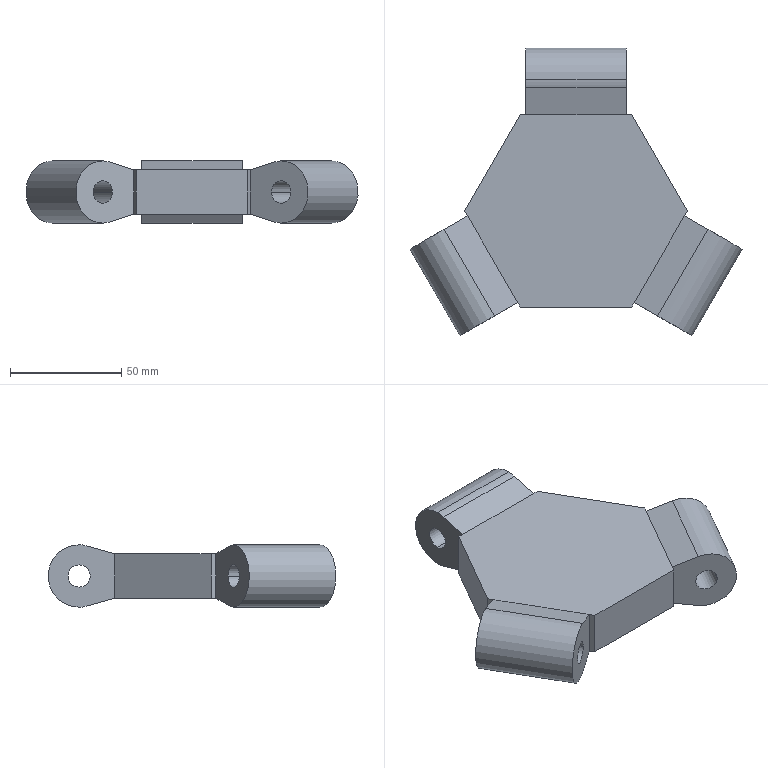Part | SolidWorks | features ICE 2, CirPattern 1, Extrusion 1 | 1 solid | 37 faces | box 149.462 x 129.437 x 28 mm | volume 213673 mm3 | plane 24 | cylinder 13 | commonest cylinder face diameters 10 x8 28 x5
STEP:
#1=CARTESIAN_POINT('',(35.776,-46.636,10.001));
#2=VERTEX_POINT('',#1);
#3=CARTESIAN_POINT('',(44.437,-51.636,10.001));
#4=VERTEX_POINT('',#3);
#5=CARTESIAN_POINT('',(40.106,-49.136,10.001));
#6=DIRECTION('',(-0.5,-0.866,0.));
#7=DIRECTION('',(0.,0.,-1.));
#8=AXIS2_PLACEMENT_3D('',#5,#6,#7);
#9=CIRCLE('',#8,5.);
#10=EDGE_CURVE('',#2,#4,#9,.T.);
#11=ORIENTED_EDGE('',*,*,#10,.T.);
#12=CARTESIAN_POINT('',(66.937,-12.665,10.001));
#13=VERTEX_POINT('',#12);
#14=CARTESIAN_POINT('',(44.437,-51.636,10.001));
#15=DIRECTION('',(0.5,0.866,0.));
#16=VECTOR('',#15,1000.);
#17=LINE('',#14,#16);
#18=EDGE_CURVE('',#4,#13,#17,.T.);
#19=ORIENTED_EDGE('',*,*,#18,.T.);
#20=CARTESIAN_POINT('',(58.276,-7.665,10.001));
#21=VERTEX_POINT('',#20);
#22=CARTESIAN_POINT('',(62.606,-10.165,10.001));
#23=DIRECTION('',(-0.5,-0.866,0.));
#24=DIRECTION('',(0.,0.,-1.));
#25=AXIS2_PLACEMENT_3D('',#22,#23,#24);
#26=CIRCLE('',#25,5.);
#27=EDGE_CURVE('',#21,#13,#26,.T.);
#28=ORIENTED_EDGE('',*,*,#27,.F.);
#29=CARTESIAN_POINT('',(35.776,-46.636,10.001));
#30=DIRECTION('',(0.5,0.866,0.));
#31=VECTOR('',#30,1000.);
#32=LINE('',#29,#31);
#33=EDGE_CURVE('',#2,#21,#32,.T.);
#34=ORIENTED_EDGE('',*,*,#33,.F.);
#35=EDGE_LOOP('',(#11,#19,#28,#34));
#36=FACE_OUTER_BOUND('',#35,.T.);
#37=CARTESIAN_POINT('',(40.106,-49.136,10.001));
#38=DIRECTION('',(0.5,0.866,0.));
#39=DIRECTION('',(-0.866,0.5,0.));
#40=AXIS2_PLACEMENT_3D('',#37,#38,#39);
#41=CYLINDRICAL_SURFACE('',#40,5.);
#42=ADVANCED_FACE('',(#36),#41,.F.);
#43=CARTESIAN_POINT('',(-58.276,-7.665,10.001));
#44=VERTEX_POINT('',#43);
#45=CARTESIAN_POINT('',(-66.937,-12.665,10.001));
#46=VERTEX_POINT('',#45);
#47=CARTESIAN_POINT('',(-62.606,-10.165,10.001));
#48=DIRECTION('',(-0.5,0.866,0.));
#49=DIRECTION('',(0.,0.,-1.));
#50=AXIS2_PLACEMENT_3D('',#47,#48,#49);
#51=CIRCLE('',#50,5.);
#52=EDGE_CURVE('',#44,#46,#51,.T.);
#53=ORIENTED_EDGE('',*,*,#52,.T.);
#54=CARTESIAN_POINT('',(-44.437,-51.636,10.001));
#55=VERTEX_POINT('',#54);
#56=CARTESIAN_POINT('',(-66.937,-12.665,10.001));
#57=DIRECTION('',(0.5,-0.866,0.));
#58=VECTOR('',#57,1000.);
#59=LINE('',#56,#58);
#60=EDGE_CURVE('',#46,#55,#59,.T.);
#61=ORIENTED_EDGE('',*,*,#60,.T.);
#62=CARTESIAN_POINT('',(-35.776,-46.636,10.001));
#63=VERTEX_POINT('',#62);
#64=CARTESIAN_POINT('',(-40.106,-49.136,10.001));
#65=DIRECTION('',(-0.5,0.866,0.));
#66=DIRECTION('',(0.,0.,-1.));
#67=AXIS2_PLACEMENT_3D('',#64,#65,#66);
#68=CIRCLE('',#67,5.);
#69=EDGE_CURVE('',#63,#55,#68,.T.);
#70=ORIENTED_EDGE('',*,*,#69,.F.);
#71=CARTESIAN_POINT('',(-58.276,-7.665,10.001));
#72=DIRECTION('',(0.5,-0.866,0.));
#73=VECTOR('',#72,1000.);
#74=LINE('',#71,#73);
#75=EDGE_CURVE('',#44,#63,#74,.T.);
#76=ORIENTED_EDGE('',*,*,#75,.F.);
#77=EDGE_LOOP('',(#53,#61,#70,#76));
#78=FACE_OUTER_BOUND('',#77,.T.);
#79=CARTESIAN_POINT('',(-62.606,-10.165,10.001));
#80=DIRECTION('',(0.5,-0.866,0.));
#81=DIRECTION('',(0.866,0.5,0.));
#82=AXIS2_PLACEMENT_3D('',#79,#80,#81);
#83=CYLINDRICAL_SURFACE('',#82,5.);
#84=ADVANCED_FACE('',(#78),#83,.F.);
#85=CARTESIAN_POINT('',(5.,0.,0.5));
#86=VERTEX_POINT('',#85);
#87=CARTESIAN_POINT('',(-5.,0.,0.5));
#88=VERTEX_POINT('',#87);
#89=CARTESIAN_POINT('',(0.,0.,0.5));
#90=DIRECTION('',(0.,0.,-1.));
#91=DIRECTION('',(-1.,0.,0.));
#92=AXIS2_PLACEMENT_3D('',#89,#90,#91);
#93=CIRCLE('',#92,5.);
#94=EDGE_CURVE('',#86,#88,#93,.T.);
#95=ORIENTED_EDGE('',*,*,#94,.F.);
#96=CARTESIAN_POINT('',(5.,0.,0.));
#97=VERTEX_POINT('',#96);
#98=CARTESIAN_POINT('',(5.,0.,0.5));
#99=DIRECTION('',(0.,0.,-1.));
#100=VECTOR('',#99,1000.);
#101=LINE('',#98,#100);
#102=EDGE_CURVE('',#86,#97,#101,.T.);
#103=ORIENTED_EDGE('',*,*,#102,.T.);
#104=CARTESIAN_POINT('',(-5.,0.,0.));
#105=VERTEX_POINT('',#104);
#106=CARTESIAN_POINT('',(0.,0.,0.));
#107=DIRECTION('',(0.,0.,-1.));
#108=DIRECTION('',(-1.,0.,0.));
#109=AXIS2_PLACEMENT_3D('',#106,#107,#108);
#110=CIRCLE('',#109,5.);
#111=EDGE_CURVE('',#97,#105,#110,.T.);
#112=ORIENTED_EDGE('',*,*,#111,.T.);
#113=CARTESIAN_POINT('',(-5.,0.,0.5));
#114=DIRECTION('',(0.,0.,-1.));
#115=VECTOR('',#114,1000.);
#116=LINE('',#113,#115);
#117=EDGE_CURVE('',#88,#105,#116,.T.);
#118=ORIENTED_EDGE('',*,*,#117,.F.);
#119=EDGE_LOOP('',(#95,#103,#112,#118));
#120=FACE_OUTER_BOUND('',#119,.T.);
#121=CARTESIAN_POINT('',(0.,0.,0.5));
#122=DIRECTION('',(0.,0.,-1.));
#123=DIRECTION('',(-1.,0.,0.));
#124=AXIS2_PLACEMENT_3D('',#121,#122,#123);
#125=CYLINDRICAL_SURFACE('',#124,5.);
#126=ADVANCED_FACE('',(#120),#125,.F.);
#127=CARTESIAN_POINT('',(22.5,59.301,15.001));
#128=VERTEX_POINT('',#127);
#129=CARTESIAN_POINT('',(22.5,59.301,5.001));
#130=VERTEX_POINT('',#129);
#131=CARTESIAN_POINT('',(22.5,59.301,10.001));
#132=DIRECTION('',(1.,0.,0.));
#133=DIRECTION('',(0.,0.,-1.));
#134=AXIS2_PLACEMENT_3D('',#131,#132,#133);
#135=CIRCLE('',#134,5.);
#136=EDGE_CURVE('',#128,#130,#135,.T.);
#137=ORIENTED_EDGE('',*,*,#136,.T.);
#138=CARTESIAN_POINT('',(-22.5,59.301,5.001));
#139=VERTEX_POINT('',#138);
#140=CARTESIAN_POINT('',(22.5,59.301,5.001));
#141=DIRECTION('',(-1.,0.,0.));
#142=VECTOR('',#141,1000.);
#143=LINE('',#140,#142);
#144=EDGE_CURVE('',#130,#139,#143,.T.);
#145=ORIENTED_EDGE('',*,*,#144,.T.);
#146=CARTESIAN_POINT('',(-22.5,59.301,15.001));
#147=VERTEX_POINT('',#146);
#148=CARTESIAN_POINT('',(-22.5,59.301,10.001));
#149=DIRECTION('',(1.,0.,0.));
#150=DIRECTION('',(0.,0.,-1.));
#151=AXIS2_PLACEMENT_3D('',#148,#149,#150);
#152=CIRCLE('',#151,5.);
#153=EDGE_CURVE('',#147,#139,#152,.T.);
#154=ORIENTED_EDGE('',*,*,#153,.F.);
#155=CARTESIAN_POINT('',(22.5,59.301,15.001));
#156=DIRECTION('',(-1.,0.,0.));
#157=VECTOR('',#156,1000.);
#158=LINE('',#155,#157);
#159=EDGE_CURVE('',#128,#147,#158,.T.);
#160=ORIENTED_EDGE('',*,*,#159,.F.);
#161=EDGE_LOOP('',(#137,#145,#154,#160));
#162=FACE_OUTER_BOUND('',#161,.T.);
#163=CARTESIAN_POINT('',(22.5,59.301,10.001));
#164=DIRECTION('',(-1.,0.,0.));
#165=DIRECTION('',(0.,0.,1.));
#166=AXIS2_PLACEMENT_3D('',#163,#164,#165);
#167=CYLINDRICAL_SURFACE('',#166,5.);
#168=ADVANCED_FACE('',(#162),#167,.F.);
#169=CARTESIAN_POINT('',(22.5,59.301,-3.999));
#170=VERTEX_POINT('',#169);
#171=CARTESIAN_POINT('',(22.5,59.301,24.001));
#172=VERTEX_POINT('',#171);
#173=CARTESIAN_POINT('',(22.5,59.301,10.001));
#174=DIRECTION('',(1.,0.,0.));
#175=DIRECTION('',(0.,0.,-1.));
#176=AXIS2_PLACEMENT_3D('',#173,#174,#175);
#177=CIRCLE('',#176,14.);
#178=EDGE_CURVE('',#170,#172,#177,.T.);
#179=ORIENTED_EDGE('',*,*,#178,.F.);
#180=CARTESIAN_POINT('',(-22.5,59.301,-3.999));
#181=VERTEX_POINT('',#180);
#182=CARTESIAN_POINT('',(22.5,59.301,-3.999));
#183=DIRECTION('',(-1.,0.,0.));
#184=VECTOR('',#183,1000.);
#185=LINE('',#182,#184);
#186=EDGE_CURVE('',#170,#181,#185,.T.);
#187=ORIENTED_EDGE('',*,*,#186,.T.);
#188=CARTESIAN_POINT('',(-22.5,59.301,24.001));
#189=VERTEX_POINT('',#188);
#190=CARTESIAN_POINT('',(-22.5,59.301,10.001));
#191=DIRECTION('',(1.,0.,0.));
#192=DIRECTION('',(0.,0.,-1.));
#193=AXIS2_PLACEMENT_3D('',#190,#191,#192);
#194=CIRCLE('',#193,14.);
#195=EDGE_CURVE('',#181,#189,#194,.T.);
#196=ORIENTED_EDGE('',*,*,#195,.T.);
#197=CARTESIAN_POINT('',(22.5,59.301,24.001));
#198=DIRECTION('',(-1.,0.,0.));
#199=VECTOR('',#198,1000.);
#200=LINE('',#197,#199);
#201=EDGE_CURVE('',#172,#189,#200,.T.);
#202=ORIENTED_EDGE('',*,*,#201,.F.);
#203=EDGE_LOOP('',(#179,#187,#196,#202));
#204=FACE_OUTER_BOUND('',#203,.T.);
#205=CARTESIAN_POINT('',(22.5,59.301,10.001));
#206=DIRECTION('',(-1.,0.,0.));
#207=DIRECTION('',(0.,0.,1.));
#208=AXIS2_PLACEMENT_3D('',#205,#206,#207);
#209=CYLINDRICAL_SURFACE('',#208,14.);
#210=ADVANCED_FACE('',(#204),#209,.T.);
#211=CARTESIAN_POINT('',(22.5,55.466,23.465));
#212=VERTEX_POINT('',#211);
#213=CARTESIAN_POINT('',(22.5,59.301,10.001));
#214=DIRECTION('',(1.,0.,0.));
#215=DIRECTION('',(0.,0.,-1.));
#216=AXIS2_PLACEMENT_3D('',#213,#214,#215);
#217=CIRCLE('',#216,14.);
#218=EDGE_CURVE('',#172,#212,#217,.T.);
#219=ORIENTED_EDGE('',*,*,#218,.F.);
#220=ORIENTED_EDGE('',*,*,#201,.T.);
#221=CARTESIAN_POINT('',(-22.5,55.466,23.465));
#222=VERTEX_POINT('',#221);
#223=CARTESIAN_POINT('',(-22.5,59.301,10.001));
#224=DIRECTION('',(1.,0.,0.));
#225=DIRECTION('',(0.,0.,-1.));
#226=AXIS2_PLACEMENT_3D('',#223,#224,#225);
#227=CIRCLE('',#226,14.);
#228=EDGE_CURVE('',#189,#222,#227,.T.);
#229=ORIENTED_EDGE('',*,*,#228,.T.);
#230=CARTESIAN_POINT('',(22.5,55.466,23.465));
#231=DIRECTION('',(-1.,0.,0.));
#232=VECTOR('',#231,1000.);
#233=LINE('',#230,#232);
#234=EDGE_CURVE('',#212,#222,#233,.T.);
#235=ORIENTED_EDGE('',*,*,#234,.F.);
#236=EDGE_LOOP('',(#219,#220,#229,#235));
#237=FACE_OUTER_BOUND('',#236,.T.);
#238=CARTESIAN_POINT('',(22.5,59.301,10.001));
#239=DIRECTION('',(-1.,0.,0.));
#240=DIRECTION('',(0.,0.,1.));
#241=AXIS2_PLACEMENT_3D('',#238,#239,#240);
#242=CYLINDRICAL_SURFACE('',#241,14.);
#243=ADVANCED_FACE('',(#237),#242,.T.);
#244=CARTESIAN_POINT('',(48.75,-2.165,20.));
#245=VERTEX_POINT('',#244);
#246=CARTESIAN_POINT('',(48.75,-2.165,0.));
#247=VERTEX_POINT('',#246);
#248=CARTESIAN_POINT('',(48.75,-2.165,20.));
#249=DIRECTION('',(0.,0.,-1.));
#250=VECTOR('',#249,1000.);
#251=LINE('',#248,#250);
#252=EDGE_CURVE('',#245,#247,#251,.T.);
#253=ORIENTED_EDGE('',*,*,#252,.T.);
#254=CARTESIAN_POINT('',(50.,0.,0.));
#255=VERTEX_POINT('',#254);
#256=CARTESIAN_POINT('',(25.,-43.301,0.));
#257=DIRECTION('',(0.5,0.866,0.));
#258=VECTOR('',#257,1000.);
#259=LINE('',#256,#258);
#260=EDGE_CURVE('',#247,#255,#259,.T.);
#261=ORIENTED_EDGE('',*,*,#260,.T.);
#262=CARTESIAN_POINT('',(50.,0.,20.));
#263=VERTEX_POINT('',#262);
#264=CARTESIAN_POINT('',(50.,0.,20.));
#265=DIRECTION('',(0.,0.,-1.));
#266=VECTOR('',#265,1000.);
#267=LINE('',#264,#266);
#268=EDGE_CURVE('',#263,#255,#267,.T.);
#269=ORIENTED_EDGE('',*,*,#268,.F.);
#270=CARTESIAN_POINT('',(25.,-43.301,20.));
#271=DIRECTION('',(0.5,0.866,0.));
#272=VECTOR('',#271,1000.);
#273=LINE('',#270,#272);
#274=EDGE_CURVE('',#245,#263,#273,.T.);
#275=ORIENTED_EDGE('',*,*,#274,.F.);
#276=EDGE_LOOP('',(#253,#261,#269,#275));
#277=FACE_OUTER_BOUND('',#276,.T.);
#278=CARTESIAN_POINT('',(25.,-43.301,20.));
#279=DIRECTION('',(-0.866,0.5,0.));
#280=DIRECTION('',(-0.5,-0.866,0.));
#281=AXIS2_PLACEMENT_3D('',#278,#279,#280);
#282=PLANE('',#281);
#283=ADVANCED_FACE('',(#277),#282,.F.);
#284=CARTESIAN_POINT('',(-26.25,-41.136,20.));
#285=VERTEX_POINT('',#284);
#286=CARTESIAN_POINT('',(-26.25,-41.136,0.));
#287=VERTEX_POINT('',#286);
#288=CARTESIAN_POINT('',(-26.25,-41.136,20.));
#289=DIRECTION('',(0.,0.,-1.));
#290=VECTOR('',#289,1000.);
#291=LINE('',#288,#290);
#292=EDGE_CURVE('',#285,#287,#291,.T.);
#293=ORIENTED_EDGE('',*,*,#292,.T.);
#294=CARTESIAN_POINT('',(-25.,-43.301,0.));
#295=VERTEX_POINT('',#294);
#296=CARTESIAN_POINT('',(-50.,0.,0.));
#297=DIRECTION('',(0.5,-0.866,0.));
#298=VECTOR('',#297,1000.);
#299=LINE('',#296,#298);
#300=EDGE_CURVE('',#287,#295,#299,.T.);
#301=ORIENTED_EDGE('',*,*,#300,.T.);
#302=CARTESIAN_POINT('',(-25.,-43.301,20.));
#303=VERTEX_POINT('',#302);
#304=CARTESIAN_POINT('',(-25.,-43.301,20.));
#305=DIRECTION('',(0.,0.,-1.));
#306=VECTOR('',#305,1000.);
#307=LINE('',#304,#306);
#308=EDGE_CURVE('',#303,#295,#307,.T.);
#309=ORIENTED_EDGE('',*,*,#308,.F.);
#310=CARTESIAN_POINT('',(-50.,0.,20.));
#311=DIRECTION('',(0.5,-0.866,0.));
#312=VECTOR('',#311,1000.);
#313=LINE('',#310,#312);
#314=EDGE_CURVE('',#285,#303,#313,.T.);
#315=ORIENTED_EDGE('',*,*,#314,.F.);
#316=EDGE_LOOP('',(#293,#301,#309,#315));
#317=FACE_OUTER_BOUND('',#316,.T.);
#318=CARTESIAN_POINT('',(-50.,0.,20.));
#319=DIRECTION('',(0.866,0.5,0.));
#320=DIRECTION('',(-0.5,0.866,0.));
#321=AXIS2_PLACEMENT_3D('',#318,#319,#320);
#322=PLANE('',#321);
#323=ADVANCED_FACE('',(#317),#322,.F.);
#324=CARTESIAN_POINT('',(22.5,43.301,20.));
#325=VERTEX_POINT('',#324);
#326=CARTESIAN_POINT('',(22.5,43.301,0.));
#327=VERTEX_POINT('',#326);
#328=CARTESIAN_POINT('',(22.5,43.301,20.));
#329=DIRECTION('',(0.,0.,-1.));
#330=VECTOR('',#329,1000.);
#331=LINE('',#328,#330);
#332=EDGE_CURVE('',#325,#327,#331,.T.);
#333=ORIENTED_EDGE('',*,*,#332,.F.);
#334=CARTESIAN_POINT('',(25.,43.301,20.));
#335=VERTEX_POINT('',#334);
#336=CARTESIAN_POINT('',(25.,43.301,20.));
#337=DIRECTION('',(-1.,0.,0.));
#338=VECTOR('',#337,1000.);
#339=LINE('',#336,#338);
#340=EDGE_CURVE('',#335,#325,#339,.T.);
#341=ORIENTED_EDGE('',*,*,#340,.F.);
#342=CARTESIAN_POINT('',(25.,43.301,0.));
#343=VERTEX_POINT('',#342);
#344=CARTESIAN_POINT('',(25.,43.301,20.));
#345=DIRECTION('',(0.,0.,-1.));
#346=VECTOR('',#345,1000.);
#347=LINE('',#344,#346);
#348=EDGE_CURVE('',#335,#343,#347,.T.);
#349=ORIENTED_EDGE('',*,*,#348,.T.);
#350=CARTESIAN_POINT('',(25.,43.301,0.));
#351=DIRECTION('',(-1.,0.,0.));
#352=VECTOR('',#351,1000.);
#353=LINE('',#350,#352);
#354=EDGE_CURVE('',#343,#327,#353,.T.);
#355=ORIENTED_EDGE('',*,*,#354,.T.);
#356=EDGE_LOOP('',(#333,#341,#349,#355));
#357=FACE_OUTER_BOUND('',#356,.T.);
#358=CARTESIAN_POINT('',(25.,43.301,20.));
#359=DIRECTION('',(0.,-1.,0.));
#360=DIRECTION('',(1.,0.,0.));
#361=AXIS2_PLACEMENT_3D('',#358,#359,#360);
#362=PLANE('',#361);
#363=ADVANCED_FACE('',(#357),#362,.F.);
#364=CARTESIAN_POINT('',(25.,-43.301,0.));
#365=VERTEX_POINT('',#364);
#366=CARTESIAN_POINT('',(26.25,-41.136,0.));
#367=VERTEX_POINT('',#366);
#368=CARTESIAN_POINT('',(25.,-43.301,0.));
#369=DIRECTION('',(0.5,0.866,0.));
#370=VECTOR('',#369,1000.);
#371=LINE('',#368,#370);
#372=EDGE_CURVE('',#365,#367,#371,.T.);
#373=ORIENTED_EDGE('',*,*,#372,.T.);
#374=CARTESIAN_POINT('',(26.25,-41.136,20.));
#375=VERTEX_POINT('',#374);
#376=CARTESIAN_POINT('',(26.25,-41.136,20.));
#377=DIRECTION('',(0.,0.,-1.));
#378=VECTOR('',#377,1000.);
#379=LINE('',#376,#378);
#380=EDGE_CURVE('',#375,#367,#379,.T.);
#381=ORIENTED_EDGE('',*,*,#380,.F.);
#382=CARTESIAN_POINT('',(25.,-43.301,20.));
#383=VERTEX_POINT('',#382);
#384=CARTESIAN_POINT('',(25.,-43.301,20.));
#385=DIRECTION('',(0.5,0.866,0.));
#386=VECTOR('',#385,1000.);
#387=LINE('',#384,#386);
#388=EDGE_CURVE('',#383,#375,#387,.T.);
#389=ORIENTED_EDGE('',*,*,#388,.F.);
#390=CARTESIAN_POINT('',(25.,-43.301,20.));
#391=DIRECTION('',(0.,0.,-1.));
#392=VECTOR('',#391,1000.);
#393=LINE('',#390,#392);
#394=EDGE_CURVE('',#383,#365,#393,.T.);
#395=ORIENTED_EDGE('',*,*,#394,.T.);
#396=EDGE_LOOP('',(#373,#381,#389,#395));
#397=FACE_OUTER_BOUND('',#396,.T.);
#398=CARTESIAN_POINT('',(25.,-43.301,20.));
#399=DIRECTION('',(-0.866,0.5,0.));
#400=DIRECTION('',(-0.5,-0.866,0.));
#401=AXIS2_PLACEMENT_3D('',#398,#399,#400);
#402=PLANE('',#401);
#403=ADVANCED_FACE('',(#397),#402,.F.);
#404=CARTESIAN_POINT('',(50.,0.,0.));
#405=DIRECTION('',(-0.5,0.866,0.));
#406=VECTOR('',#405,1000.);
#407=LINE('',#404,#406);
#408=EDGE_CURVE('',#255,#343,#407,.T.);
#409=ORIENTED_EDGE('',*,*,#408,.T.);
#410=ORIENTED_EDGE('',*,*,#348,.F.);
#411=CARTESIAN_POINT('',(50.,0.,20.));
#412=DIRECTION('',(-0.5,0.866,0.));
#413=VECTOR('',#412,1000.);
#414=LINE('',#411,#413);
#415=EDGE_CURVE('',#263,#335,#414,.T.);
#416=ORIENTED_EDGE('',*,*,#415,.F.);
#417=ORIENTED_EDGE('',*,*,#268,.T.);
#418=EDGE_LOOP('',(#409,#410,#416,#417));
#419=FACE_OUTER_BOUND('',#418,.T.);
#420=CARTESIAN_POINT('',(50.,0.,20.));
#421=DIRECTION('',(-0.866,-0.5,0.));
#422=DIRECTION('',(0.5,-0.866,0.));
#423=AXIS2_PLACEMENT_3D('',#420,#421,#422);
#424=PLANE('',#423);
#425=ADVANCED_FACE('',(#419),#424,.F.);
#426=CARTESIAN_POINT('',(-22.5,43.301,20.));
#427=VERTEX_POINT('',#426);
#428=CARTESIAN_POINT('',(-25.,43.301,20.));
#429=VERTEX_POINT('',#428);
#430=CARTESIAN_POINT('',(25.,43.301,20.));
#431=DIRECTION('',(-1.,0.,0.));
#432=VECTOR('',#431,1000.);
#433=LINE('',#430,#432);
#434=EDGE_CURVE('',#427,#429,#433,.T.);
#435=ORIENTED_EDGE('',*,*,#434,.F.);
#436=CARTESIAN_POINT('',(-22.5,43.301,0.));
#437=VERTEX_POINT('',#436);
#438=CARTESIAN_POINT('',(-22.5,43.301,20.));
#439=DIRECTION('',(0.,0.,-1.));
#440=VECTOR('',#439,1000.);
#441=LINE('',#438,#440);
#442=EDGE_CURVE('',#427,#437,#441,.T.);
#443=ORIENTED_EDGE('',*,*,#442,.T.);
#444=CARTESIAN_POINT('',(-25.,43.301,0.));
#445=VERTEX_POINT('',#444);
#446=CARTESIAN_POINT('',(25.,43.301,0.));
#447=DIRECTION('',(-1.,0.,0.));
#448=VECTOR('',#447,1000.);
#449=LINE('',#446,#448);
#450=EDGE_CURVE('',#437,#445,#449,.T.);
#451=ORIENTED_EDGE('',*,*,#450,.T.);
#452=CARTESIAN_POINT('',(-25.,43.301,20.));
#453=DIRECTION('',(0.,0.,-1.));
#454=VECTOR('',#453,1000.);
#455=LINE('',#452,#454);
#456=EDGE_CURVE('',#429,#445,#455,.T.);
#457=ORIENTED_EDGE('',*,*,#456,.F.);
#458=EDGE_LOOP('',(#435,#443,#451,#457));
#459=FACE_OUTER_BOUND('',#458,.T.);
#460=CARTESIAN_POINT('',(25.,43.301,20.));
#461=DIRECTION('',(0.,-1.,0.));
#462=DIRECTION('',(1.,0.,0.));
#463=AXIS2_PLACEMENT_3D('',#460,#461,#462);
#464=PLANE('',#463);
#465=ADVANCED_FACE('',(#459),#464,.F.);
#466=CARTESIAN_POINT('',(-50.,0.,0.));
#467=VERTEX_POINT('',#466);
#468=CARTESIAN_POINT('',(-25.,43.301,0.));
#469=DIRECTION('',(-0.5,-0.866,0.));
#470=VECTOR('',#469,1000.);
#471=LINE('',#468,#470);
#472=EDGE_CURVE('',#445,#467,#471,.T.);
#473=ORIENTED_EDGE('',*,*,#472,.T.);
#474=CARTESIAN_POINT('',(-50.,0.,20.));
#475=VERTEX_POINT('',#474);
#476=CARTESIAN_POINT('',(-50.,0.,20.));
#477=DIRECTION('',(0.,0.,-1.));
#478=VECTOR('',#477,1000.);
#479=LINE('',#476,#478);
#480=EDGE_CURVE('',#475,#467,#479,.T.);
#481=ORIENTED_EDGE('',*,*,#480,.F.);
#482=CARTESIAN_POINT('',(-25.,43.301,20.));
#483=DIRECTION('',(-0.5,-0.866,0.));
#484=VECTOR('',#483,1000.);
#485=LINE('',#482,#484);
#486=EDGE_CURVE('',#429,#475,#485,.T.);
#487=ORIENTED_EDGE('',*,*,#486,.F.);
#488=ORIENTED_EDGE('',*,*,#456,.T.);
#489=EDGE_LOOP('',(#473,#481,#487,#488));
#490=FACE_OUTER_BOUND('',#489,.T.);
#491=CARTESIAN_POINT('',(-25.,43.301,20.));
#492=DIRECTION('',(0.866,-0.5,0.));
#493=DIRECTION('',(0.5,0.866,0.));
#494=AXIS2_PLACEMENT_3D('',#491,#492,#493);
#495=PLANE('',#494);
#496=ADVANCED_FACE('',(#490),#495,.F.);
#497=CARTESIAN_POINT('',(-48.75,-2.165,0.));
#498=VERTEX_POINT('',#497);
#499=CARTESIAN_POINT('',(-50.,0.,0.));
#500=DIRECTION('',(0.5,-0.866,0.));
#501=VECTOR('',#500,1000.);
#502=LINE('',#499,#501);
#503=EDGE_CURVE('',#467,#498,#502,.T.);
#504=ORIENTED_EDGE('',*,*,#503,.T.);
#505=CARTESIAN_POINT('',(-48.75,-2.165,20.));
#506=VERTEX_POINT('',#505);
#507=CARTESIAN_POINT('',(-48.75,-2.165,20.));
#508=DIRECTION('',(0.,0.,-1.));
#509=VECTOR('',#508,1000.);
#510=LINE('',#507,#509);
#511=EDGE_CURVE('',#506,#498,#510,.T.);
#512=ORIENTED_EDGE('',*,*,#511,.F.);
#513=CARTESIAN_POINT('',(-50.,0.,20.));
#514=DIRECTION('',(0.5,-0.866,0.));
#515=VECTOR('',#514,1000.);
#516=LINE('',#513,#515);
#517=EDGE_CURVE('',#475,#506,#516,.T.);
#518=ORIENTED_EDGE('',*,*,#517,.F.);
#519=ORIENTED_EDGE('',*,*,#480,.T.);
#520=EDGE_LOOP('',(#504,#512,#518,#519));
#521=FACE_OUTER_BOUND('',#520,.T.);
#522=CARTESIAN_POINT('',(-50.,0.,20.));
#523=DIRECTION('',(0.866,0.5,0.));
#524=DIRECTION('',(-0.5,0.866,0.));
#525=AXIS2_PLACEMENT_3D('',#522,#523,#524);
#526=PLANE('',#525);
#527=ADVANCED_FACE('',(#521),#526,.F.);
#528=CARTESIAN_POINT('',(-25.,-43.301,0.));
#529=DIRECTION('',(1.,0.,0.));
#530=VECTOR('',#529,1000.);
#531=LINE('',#528,#530);
#532=EDGE_CURVE('',#295,#365,#531,.T.);
#533=ORIENTED_EDGE('',*,*,#532,.T.);
#534=ORIENTED_EDGE('',*,*,#394,.F.);
#535=CARTESIAN_POINT('',(-25.,-43.301,20.));
#536=DIRECTION('',(1.,0.,0.));
#537=VECTOR('',#536,1000.);
#538=LINE('',#535,#537);
#539=EDGE_CURVE('',#303,#383,#538,.T.);
#540=ORIENTED_EDGE('',*,*,#539,.F.);
#541=ORIENTED_EDGE('',*,*,#308,.T.);
#542=EDGE_LOOP('',(#533,#534,#540,#541));
#543=FACE_OUTER_BOUND('',#542,.T.);
#544=CARTESIAN_POINT('',(-25.,-43.301,20.));
#545=DIRECTION('',(0.,1.,0.));
#546=DIRECTION('',(-1.,0.,0.));
#547=AXIS2_PLACEMENT_3D('',#544,#545,#546);
#548=PLANE('',#547);
#549=ADVANCED_FACE('',(#543),#548,.F.);
#550=ORIENTED_EDGE('',*,*,#388,.T.);
#551=CARTESIAN_POINT('',(26.25,-41.136,20.));
#552=DIRECTION('',(0.5,0.866,0.));
#553=VECTOR('',#552,1000.);
#554=LINE('',#551,#553);
#555=EDGE_CURVE('',#375,#245,#554,.T.);
#556=ORIENTED_EDGE('',*,*,#555,.T.);
#557=ORIENTED_EDGE('',*,*,#274,.T.);
#558=ORIENTED_EDGE('',*,*,#415,.T.);
#559=ORIENTED_EDGE('',*,*,#340,.T.);
#560=CARTESIAN_POINT('',(22.5,43.301,20.));
#561=DIRECTION('',(-1.,0.,0.));
#562=VECTOR('',#561,1000.);
#563=LINE('',#560,#562);
#564=EDGE_CURVE('',#325,#427,#563,.T.);
#565=ORIENTED_EDGE('',*,*,#564,.T.);
#566=ORIENTED_EDGE('',*,*,#434,.T.);
#567=ORIENTED_EDGE('',*,*,#486,.T.);
#568=ORIENTED_EDGE('',*,*,#517,.T.);
#569=CARTESIAN_POINT('',(-48.75,-2.165,20.));
#570=DIRECTION('',(0.5,-0.866,0.));
#571=VECTOR('',#570,1000.);
#572=LINE('',#569,#571);
#573=EDGE_CURVE('',#506,#285,#572,.T.);
#574=ORIENTED_EDGE('',*,*,#573,.T.);
#575=ORIENTED_EDGE('',*,*,#314,.T.);
#576=ORIENTED_EDGE('',*,*,#539,.T.);
#577=EDGE_LOOP('',(#550,#556,#557,#558,#559,#565,#566,#567,#568,#574,#575,#576));
#578=FACE_OUTER_BOUND('',#577,.T.);
#579=CARTESIAN_POINT('',(0.,0.,20.));
#580=DIRECTION('',(0.,0.,1.));
#581=DIRECTION('',(1.,0.,0.));
#582=AXIS2_PLACEMENT_3D('',#579,#580,#581);
#583=PLANE('',#582);
#584=ADVANCED_FACE('',(#578),#583,.T.);
#585=CARTESIAN_POINT('',(0.,0.,0.));
#586=DIRECTION('',(0.,0.,-1.));
#587=DIRECTION('',(-1.,0.,0.));
#588=AXIS2_PLACEMENT_3D('',#585,#586,#587);
#589=CIRCLE('',#588,5.);
#590=EDGE_CURVE('',#105,#97,#589,.T.);
#591=ORIENTED_EDGE('',*,*,#590,.F.);
#592=ORIENTED_EDGE('',*,*,#111,.F.);
#593=EDGE_LOOP('',(#591,#592));
#594=FACE_BOUND('',#593,.T.);
#595=ORIENTED_EDGE('',*,*,#372,.F.);
#596=ORIENTED_EDGE('',*,*,#532,.F.);
#597=ORIENTED_EDGE('',*,*,#300,.F.);
#598=CARTESIAN_POINT('',(-48.75,-2.165,0.));
#599=DIRECTION('',(0.5,-0.866,0.));
#600=VECTOR('',#599,1000.);
#601=LINE('',#598,#600);
#602=EDGE_CURVE('',#498,#287,#601,.T.);
#603=ORIENTED_EDGE('',*,*,#602,.F.);
#604=ORIENTED_EDGE('',*,*,#503,.F.);
#605=ORIENTED_EDGE('',*,*,#472,.F.);
#606=ORIENTED_EDGE('',*,*,#450,.F.);
#607=CARTESIAN_POINT('',(22.5,43.301,0.));
#608=DIRECTION('',(-1.,0.,0.));
#609=VECTOR('',#608,1000.);
#610=LINE('',#607,#609);
#611=EDGE_CURVE('',#327,#437,#610,.T.);
#612=ORIENTED_EDGE('',*,*,#611,.F.);
#613=ORIENTED_EDGE('',*,*,#354,.F.);
#614=ORIENTED_EDGE('',*,*,#408,.F.);
#615=ORIENTED_EDGE('',*,*,#260,.F.);
#616=CARTESIAN_POINT('',(26.25,-41.136,0.));
#617=DIRECTION('',(0.5,0.866,0.));
#618=VECTOR('',#617,1000.);
#619=LINE('',#616,#618);
#620=EDGE_CURVE('',#367,#247,#619,.T.);
#621=ORIENTED_EDGE('',*,*,#620,.F.);
#622=EDGE_LOOP('',(#595,#596,#597,#603,#604,#605,#606,#612,#613,#614,#615,#621));
#623=FACE_OUTER_BOUND('',#622,.T.);
#624=CARTESIAN_POINT('',(0.,0.,0.));
#625=DIRECTION('',(0.,0.,1.));
#626=DIRECTION('',(1.,0.,0.));
#627=AXIS2_PLACEMENT_3D('',#624,#625,#626);
#628=PLANE('',#627);
#629=ADVANCED_FACE('',(#594,#623),#628,.F.);
#630=ORIENTED_EDGE('',*,*,#332,.T.);
#631=CARTESIAN_POINT('',(22.5,55.467,-3.464));
#632=VERTEX_POINT('',#631);
#633=CARTESIAN_POINT('',(22.5,43.301,0.));
#634=DIRECTION('',(0.,0.9618,-0.2738));
#635=VECTOR('',#634,1000.);
#636=LINE('',#633,#635);
#637=EDGE_CURVE('',#327,#632,#636,.T.);
#638=ORIENTED_EDGE('',*,*,#637,.T.);
#639=CARTESIAN_POINT('',(22.5,59.301,10.001));
#640=DIRECTION('',(1.,0.,0.));
#641=DIRECTION('',(0.,0.,-1.));
#642=AXIS2_PLACEMENT_3D('',#639,#640,#641);
#643=CIRCLE('',#642,14.);
#644=EDGE_CURVE('',#632,#170,#643,.T.);
#645=ORIENTED_EDGE('',*,*,#644,.T.);
#646=ORIENTED_EDGE('',*,*,#178,.T.);
#647=ORIENTED_EDGE('',*,*,#218,.T.);
#648=CARTESIAN_POINT('',(22.5,43.301,20.));
#649=DIRECTION('',(0.,-0.9617,-0.274));
#650=VECTOR('',#649,1000.);
#651=LINE('',#648,#650);
#652=EDGE_CURVE('',#212,#325,#651,.T.);
#653=ORIENTED_EDGE('',*,*,#652,.T.);
#654=EDGE_LOOP('',(#630,#638,#645,#646,#647,#653));
#655=FACE_OUTER_BOUND('',#654,.T.);
#656=ORIENTED_EDGE('',*,*,#136,.F.);
#657=CARTESIAN_POINT('',(22.5,59.301,10.001));
#658=DIRECTION('',(1.,0.,0.));
#659=DIRECTION('',(0.,0.,-1.));
#660=AXIS2_PLACEMENT_3D('',#657,#658,#659);
#661=CIRCLE('',#660,5.);
#662=EDGE_CURVE('',#130,#128,#661,.T.);
#663=ORIENTED_EDGE('',*,*,#662,.F.);
#664=EDGE_LOOP('',(#656,#663));
#665=FACE_BOUND('',#664,.T.);
#666=CARTESIAN_POINT('',(22.5,59.301,10.001));
#667=DIRECTION('',(1.,0.,0.));
#668=DIRECTION('',(0.,0.,-1.));
#669=AXIS2_PLACEMENT_3D('',#666,#667,#668);
#670=PLANE('',#669);
#671=ADVANCED_FACE('',(#655,#665),#670,.T.);
#672=ORIENTED_EDGE('',*,*,#442,.F.);
#673=CARTESIAN_POINT('',(-22.5,43.301,20.));
#674=DIRECTION('',(0.,-0.9617,-0.274));
#675=VECTOR('',#674,1000.);
#676=LINE('',#673,#675);
#677=EDGE_CURVE('',#222,#427,#676,.T.);
#678=ORIENTED_EDGE('',*,*,#677,.F.);
#679=ORIENTED_EDGE('',*,*,#228,.F.);
#680=ORIENTED_EDGE('',*,*,#195,.F.);
#681=CARTESIAN_POINT('',(-22.5,55.467,-3.464));
#682=VERTEX_POINT('',#681);
#683=CARTESIAN_POINT('',(-22.5,59.301,10.001));
#684=DIRECTION('',(1.,0.,0.));
#685=DIRECTION('',(0.,0.,-1.));
#686=AXIS2_PLACEMENT_3D('',#683,#684,#685);
#687=CIRCLE('',#686,14.);
#688=EDGE_CURVE('',#682,#181,#687,.T.);
#689=ORIENTED_EDGE('',*,*,#688,.F.);
#690=CARTESIAN_POINT('',(-22.5,43.301,0.));
#691=DIRECTION('',(0.,0.9618,-0.2738));
#692=VECTOR('',#691,1000.);
#693=LINE('',#690,#692);
#694=EDGE_CURVE('',#437,#682,#693,.T.);
#695=ORIENTED_EDGE('',*,*,#694,.F.);
#696=EDGE_LOOP('',(#672,#678,#679,#680,#689,#695));
#697=FACE_OUTER_BOUND('',#696,.T.);
#698=ORIENTED_EDGE('',*,*,#153,.T.);
#699=CARTESIAN_POINT('',(-22.5,59.301,10.001));
#700=DIRECTION('',(1.,0.,0.));
#701=DIRECTION('',(0.,0.,-1.));
#702=AXIS2_PLACEMENT_3D('',#699,#700,#701);
#703=CIRCLE('',#702,5.);
#704=EDGE_CURVE('',#139,#147,#703,.T.);
#705=ORIENTED_EDGE('',*,*,#704,.T.);
#706=EDGE_LOOP('',(#698,#705));
#707=FACE_BOUND('',#706,.T.);
#708=CARTESIAN_POINT('',(-22.5,59.301,10.001));
#709=DIRECTION('',(1.,0.,0.));
#710=DIRECTION('',(0.,0.,-1.));
#711=AXIS2_PLACEMENT_3D('',#708,#709,#710);
#712=PLANE('',#711);
#713=ADVANCED_FACE('',(#697,#707),#712,.F.);
#714=ORIENTED_EDGE('',*,*,#694,.T.);
#715=CARTESIAN_POINT('',(22.5,55.467,-3.464));
#716=DIRECTION('',(-1.,0.,0.));
#717=VECTOR('',#716,1000.);
#718=LINE('',#715,#717);
#719=EDGE_CURVE('',#632,#682,#718,.T.);
#720=ORIENTED_EDGE('',*,*,#719,.F.);
#721=ORIENTED_EDGE('',*,*,#637,.F.);
#722=ORIENTED_EDGE('',*,*,#611,.T.);
#723=EDGE_LOOP('',(#714,#720,#721,#722));
#724=FACE_OUTER_BOUND('',#723,.T.);
#725=CARTESIAN_POINT('',(22.5,43.301,0.));
#726=DIRECTION('',(0.,0.2738,0.9618));
#727=DIRECTION('',(0.,-0.9618,0.2738));
#728=AXIS2_PLACEMENT_3D('',#725,#726,#727);
#729=PLANE('',#728);
#730=ADVANCED_FACE('',(#724),#729,.F.);
#731=ORIENTED_EDGE('',*,*,#186,.F.);
#732=ORIENTED_EDGE('',*,*,#644,.F.);
#733=ORIENTED_EDGE('',*,*,#719,.T.);
#734=ORIENTED_EDGE('',*,*,#688,.T.);
#735=EDGE_LOOP('',(#731,#732,#733,#734));
#736=FACE_OUTER_BOUND('',#735,.T.);
#737=CARTESIAN_POINT('',(22.5,59.301,10.001));
#738=DIRECTION('',(-1.,0.,0.));
#739=DIRECTION('',(0.,0.,1.));
#740=AXIS2_PLACEMENT_3D('',#737,#738,#739);
#741=CYLINDRICAL_SURFACE('',#740,14.);
#742=ADVANCED_FACE('',(#736),#741,.T.);
#743=ORIENTED_EDGE('',*,*,#677,.T.);
#744=ORIENTED_EDGE('',*,*,#564,.F.);
#745=ORIENTED_EDGE('',*,*,#652,.F.);
#746=ORIENTED_EDGE('',*,*,#234,.T.);
#747=EDGE_LOOP('',(#743,#744,#745,#746));
#748=FACE_OUTER_BOUND('',#747,.T.);
#749=CARTESIAN_POINT('',(22.5,43.301,20.));
#750=DIRECTION('',(0.,0.274,-0.9617));
#751=DIRECTION('',(0.,0.9617,0.274));
#752=AXIS2_PLACEMENT_3D('',#749,#750,#751);
#753=PLANE('',#752);
#754=ADVANCED_FACE('',(#748),#753,.F.);
#755=ORIENTED_EDGE('',*,*,#144,.F.);
#756=ORIENTED_EDGE('',*,*,#662,.T.);
#757=ORIENTED_EDGE('',*,*,#159,.T.);
#758=ORIENTED_EDGE('',*,*,#704,.F.);
#759=EDGE_LOOP('',(#755,#756,#757,#758));
#760=FACE_OUTER_BOUND('',#759,.T.);
#761=CARTESIAN_POINT('',(22.5,59.301,10.001));
#762=DIRECTION('',(-1.,0.,0.));
#763=DIRECTION('',(0.,0.,1.));
#764=AXIS2_PLACEMENT_3D('',#761,#762,#763);
#765=CYLINDRICAL_SURFACE('',#764,5.);
#766=ADVANCED_FACE('',(#760),#765,.F.);
#767=ORIENTED_EDGE('',*,*,#102,.F.);
#768=CARTESIAN_POINT('',(0.,0.,0.5));
#769=DIRECTION('',(0.,0.,-1.));
#770=DIRECTION('',(-1.,0.,0.));
#771=AXIS2_PLACEMENT_3D('',#768,#769,#770);
#772=CIRCLE('',#771,5.);
#773=EDGE_CURVE('',#88,#86,#772,.T.);
#774=ORIENTED_EDGE('',*,*,#773,.F.);
#775=ORIENTED_EDGE('',*,*,#117,.T.);
#776=ORIENTED_EDGE('',*,*,#590,.T.);
#777=EDGE_LOOP('',(#767,#774,#775,#776));
#778=FACE_OUTER_BOUND('',#777,.T.);
#779=CARTESIAN_POINT('',(0.,0.,0.5));
#780=DIRECTION('',(0.,0.,-1.));
#781=DIRECTION('',(-1.,0.,0.));
#782=AXIS2_PLACEMENT_3D('',#779,#780,#781);
#783=CYLINDRICAL_SURFACE('',#782,5.);
#784=ADVANCED_FACE('',(#778),#783,.F.);
#785=ORIENTED_EDGE('',*,*,#773,.T.);
#786=ORIENTED_EDGE('',*,*,#94,.T.);
#787=EDGE_LOOP('',(#785,#786));
#788=FACE_OUTER_BOUND('',#787,.T.);
#789=CARTESIAN_POINT('',(0.,0.,0.5));
#790=DIRECTION('',(0.,0.,-1.));
#791=DIRECTION('',(-1.,0.,0.));
#792=AXIS2_PLACEMENT_3D('',#789,#790,#791);
#793=PLANE('',#792);
#794=ADVANCED_FACE('',(#788),#793,.T.);
#795=ORIENTED_EDGE('',*,*,#511,.T.);
#796=CARTESIAN_POINT('',(-59.286,-8.248,-3.464));
#797=VERTEX_POINT('',#796);
#798=CARTESIAN_POINT('',(-48.75,-2.165,0.));
#799=DIRECTION('',(-0.8329,-0.4809,-0.2738));
#800=VECTOR('',#799,1000.);
#801=LINE('',#798,#800);
#802=EDGE_CURVE('',#498,#797,#801,.T.);
#803=ORIENTED_EDGE('',*,*,#802,.T.);
#804=CARTESIAN_POINT('',(-59.285,-8.247,23.465));
#805=VERTEX_POINT('',#804);
#806=CARTESIAN_POINT('',(-62.606,-10.165,10.001));
#807=DIRECTION('',(-0.5,0.866,0.));
#808=DIRECTION('',(0.,0.,-1.));
#809=AXIS2_PLACEMENT_3D('',#806,#807,#808);
#810=CIRCLE('',#809,14.);
#811=EDGE_CURVE('',#797,#805,#810,.T.);
#812=ORIENTED_EDGE('',*,*,#811,.T.);
#813=CARTESIAN_POINT('',(-48.75,-2.165,20.));
#814=DIRECTION('',(0.8329,0.4809,-0.274));
#815=VECTOR('',#814,1000.);
#816=LINE('',#813,#815);
#817=EDGE_CURVE('',#805,#506,#816,.T.);
#818=ORIENTED_EDGE('',*,*,#817,.T.);
#819=EDGE_LOOP('',(#795,#803,#812,#818));
#820=FACE_OUTER_BOUND('',#819,.T.);
#821=ORIENTED_EDGE('',*,*,#52,.F.);
#822=CARTESIAN_POINT('',(-62.606,-10.165,10.001));
#823=DIRECTION('',(-0.5,0.866,0.));
#824=DIRECTION('',(0.,0.,-1.));
#825=AXIS2_PLACEMENT_3D('',#822,#823,#824);
#826=CIRCLE('',#825,5.);
#827=EDGE_CURVE('',#46,#44,#826,.T.);
#828=ORIENTED_EDGE('',*,*,#827,.F.);
#829=EDGE_LOOP('',(#821,#828));
#830=FACE_BOUND('',#829,.T.);
#831=CARTESIAN_POINT('',(-62.606,-10.165,10.001));
#832=DIRECTION('',(-0.5,0.866,0.));
#833=DIRECTION('',(0.,0.,-1.));
#834=AXIS2_PLACEMENT_3D('',#831,#832,#833);
#835=PLANE('',#834);
#836=ADVANCED_FACE('',(#820,#830),#835,.T.);
#837=ORIENTED_EDGE('',*,*,#292,.F.);
#838=CARTESIAN_POINT('',(-36.785,-47.219,23.465));
#839=VERTEX_POINT('',#838);
#840=CARTESIAN_POINT('',(-26.25,-41.136,20.));
#841=DIRECTION('',(0.8329,0.4809,-0.274));
#842=VECTOR('',#841,1000.);
#843=LINE('',#840,#842);
#844=EDGE_CURVE('',#839,#285,#843,.T.);
#845=ORIENTED_EDGE('',*,*,#844,.F.);
#846=CARTESIAN_POINT('',(-36.786,-47.219,-3.464));
#847=VERTEX_POINT('',#846);
#848=CARTESIAN_POINT('',(-40.106,-49.136,10.001));
#849=DIRECTION('',(-0.5,0.866,0.));
#850=DIRECTION('',(0.,0.,-1.));
#851=AXIS2_PLACEMENT_3D('',#848,#849,#850);
#852=CIRCLE('',#851,14.);
#853=EDGE_CURVE('',#847,#839,#852,.T.);
#854=ORIENTED_EDGE('',*,*,#853,.F.);
#855=CARTESIAN_POINT('',(-26.25,-41.136,0.));
#856=DIRECTION('',(-0.8329,-0.4809,-0.2738));
#857=VECTOR('',#856,1000.);
#858=LINE('',#855,#857);
#859=EDGE_CURVE('',#287,#847,#858,.T.);
#860=ORIENTED_EDGE('',*,*,#859,.F.);
#861=EDGE_LOOP('',(#837,#845,#854,#860));
#862=FACE_OUTER_BOUND('',#861,.T.);
#863=ORIENTED_EDGE('',*,*,#69,.T.);
#864=CARTESIAN_POINT('',(-40.106,-49.136,10.001));
#865=DIRECTION('',(-0.5,0.866,0.));
#866=DIRECTION('',(0.,0.,-1.));
#867=AXIS2_PLACEMENT_3D('',#864,#865,#866);
#868=CIRCLE('',#867,5.);
#869=EDGE_CURVE('',#55,#63,#868,.T.);
#870=ORIENTED_EDGE('',*,*,#869,.T.);
#871=EDGE_LOOP('',(#863,#870));
#872=FACE_BOUND('',#871,.T.);
#873=CARTESIAN_POINT('',(-40.106,-49.136,10.001));
#874=DIRECTION('',(-0.5,0.866,0.));
#875=DIRECTION('',(0.,0.,-1.));
#876=AXIS2_PLACEMENT_3D('',#873,#874,#875);
#877=PLANE('',#876);
#878=ADVANCED_FACE('',(#862,#872),#877,.F.);
#879=ORIENTED_EDGE('',*,*,#859,.T.);
#880=CARTESIAN_POINT('',(-59.286,-8.248,-3.464));
#881=DIRECTION('',(0.5,-0.866,0.));
#882=VECTOR('',#881,1000.);
#883=LINE('',#880,#882);
#884=EDGE_CURVE('',#797,#847,#883,.T.);
#885=ORIENTED_EDGE('',*,*,#884,.F.);
#886=ORIENTED_EDGE('',*,*,#802,.F.);
#887=ORIENTED_EDGE('',*,*,#602,.T.);
#888=EDGE_LOOP('',(#879,#885,#886,#887));
#889=FACE_OUTER_BOUND('',#888,.T.);
#890=CARTESIAN_POINT('',(-48.75,-2.165,0.));
#891=DIRECTION('',(-0.2372,-0.1369,0.9618));
#892=DIRECTION('',(0.9709,0.,0.2394));
#893=AXIS2_PLACEMENT_3D('',#890,#891,#892);
#894=PLANE('',#893);
#895=ADVANCED_FACE('',(#889),#894,.F.);
#896=ORIENTED_EDGE('',*,*,#853,.T.);
#897=CARTESIAN_POINT('',(-59.285,-8.247,23.465));
#898=DIRECTION('',(0.5,-0.866,0.));
#899=VECTOR('',#898,1000.);
#900=LINE('',#897,#899);
#901=EDGE_CURVE('',#805,#839,#900,.T.);
#902=ORIENTED_EDGE('',*,*,#901,.F.);
#903=ORIENTED_EDGE('',*,*,#811,.F.);
#904=ORIENTED_EDGE('',*,*,#884,.T.);
#905=EDGE_LOOP('',(#896,#902,#903,#904));
#906=FACE_OUTER_BOUND('',#905,.T.);
#907=CARTESIAN_POINT('',(-62.606,-10.165,10.001));
#908=DIRECTION('',(0.5,-0.866,0.));
#909=DIRECTION('',(0.866,0.5,0.));
#910=AXIS2_PLACEMENT_3D('',#907,#908,#909);
#911=CYLINDRICAL_SURFACE('',#910,14.);
#912=ADVANCED_FACE('',(#906),#911,.T.);
#913=ORIENTED_EDGE('',*,*,#844,.T.);
#914=ORIENTED_EDGE('',*,*,#573,.F.);
#915=ORIENTED_EDGE('',*,*,#817,.F.);
#916=ORIENTED_EDGE('',*,*,#901,.T.);
#917=EDGE_LOOP('',(#913,#914,#915,#916));
#918=FACE_OUTER_BOUND('',#917,.T.);
#919=CARTESIAN_POINT('',(-48.75,-2.165,20.));
#920=DIRECTION('',(-0.2373,-0.137,-0.9617));
#921=DIRECTION('',(-0.9709,0.,0.2395));
#922=AXIS2_PLACEMENT_3D('',#919,#920,#921);
#923=PLANE('',#922);
#924=ADVANCED_FACE('',(#918),#923,.F.);
#925=ORIENTED_EDGE('',*,*,#60,.F.);
#926=ORIENTED_EDGE('',*,*,#827,.T.);
#927=ORIENTED_EDGE('',*,*,#75,.T.);
#928=ORIENTED_EDGE('',*,*,#869,.F.);
#929=EDGE_LOOP('',(#925,#926,#927,#928));
#930=FACE_OUTER_BOUND('',#929,.T.);
#931=CARTESIAN_POINT('',(-62.606,-10.165,10.001));
#932=DIRECTION('',(0.5,-0.866,0.));
#933=DIRECTION('',(0.866,0.5,0.));
#934=AXIS2_PLACEMENT_3D('',#931,#932,#933);
#935=CYLINDRICAL_SURFACE('',#934,5.);
#936=ADVANCED_FACE('',(#930),#935,.F.);
#937=ORIENTED_EDGE('',*,*,#380,.T.);
#938=CARTESIAN_POINT('',(36.786,-47.219,-3.464));
#939=VERTEX_POINT('',#938);
#940=CARTESIAN_POINT('',(26.25,-41.136,0.));
#941=DIRECTION('',(0.8329,-0.4809,-0.2738));
#942=VECTOR('',#941,1000.);
#943=LINE('',#940,#942);
#944=EDGE_CURVE('',#367,#939,#943,.T.);
#945=ORIENTED_EDGE('',*,*,#944,.T.);
#946=CARTESIAN_POINT('',(36.785,-47.219,23.465));
#947=VERTEX_POINT('',#946);
#948=CARTESIAN_POINT('',(40.106,-49.136,10.001));
#949=DIRECTION('',(-0.5,-0.866,0.));
#950=DIRECTION('',(0.,0.,-1.));
#951=AXIS2_PLACEMENT_3D('',#948,#949,#950);
#952=CIRCLE('',#951,14.);
#953=EDGE_CURVE('',#939,#947,#952,.T.);
#954=ORIENTED_EDGE('',*,*,#953,.T.);
#955=CARTESIAN_POINT('',(26.25,-41.136,20.));
#956=DIRECTION('',(-0.8329,0.4809,-0.274));
#957=VECTOR('',#956,1000.);
#958=LINE('',#955,#957);
#959=EDGE_CURVE('',#947,#375,#958,.T.);
#960=ORIENTED_EDGE('',*,*,#959,.T.);
#961=EDGE_LOOP('',(#937,#945,#954,#960));
#962=FACE_OUTER_BOUND('',#961,.T.);
#963=ORIENTED_EDGE('',*,*,#10,.F.);
#964=CARTESIAN_POINT('',(40.106,-49.136,10.001));
#965=DIRECTION('',(-0.5,-0.866,0.));
#966=DIRECTION('',(0.,0.,-1.));
#967=AXIS2_PLACEMENT_3D('',#964,#965,#966);
#968=CIRCLE('',#967,5.);
#969=EDGE_CURVE('',#4,#2,#968,.T.);
#970=ORIENTED_EDGE('',*,*,#969,.F.);
#971=EDGE_LOOP('',(#963,#970));
#972=FACE_BOUND('',#971,.T.);
#973=CARTESIAN_POINT('',(40.106,-49.136,10.001));
#974=DIRECTION('',(-0.5,-0.866,0.));
#975=DIRECTION('',(0.,0.,-1.));
#976=AXIS2_PLACEMENT_3D('',#973,#974,#975);
#977=PLANE('',#976);
#978=ADVANCED_FACE('',(#962,#972),#977,.T.);
#979=ORIENTED_EDGE('',*,*,#252,.F.);
#980=CARTESIAN_POINT('',(59.285,-8.247,23.465));
#981=VERTEX_POINT('',#980);
#982=CARTESIAN_POINT('',(48.75,-2.165,20.));
#983=DIRECTION('',(-0.8329,0.4809,-0.274));
#984=VECTOR('',#983,1000.);
#985=LINE('',#982,#984);
#986=EDGE_CURVE('',#981,#245,#985,.T.);
#987=ORIENTED_EDGE('',*,*,#986,.F.);
#988=CARTESIAN_POINT('',(59.286,-8.248,-3.464));
#989=VERTEX_POINT('',#988);
#990=CARTESIAN_POINT('',(62.606,-10.165,10.001));
#991=DIRECTION('',(-0.5,-0.866,0.));
#992=DIRECTION('',(0.,0.,-1.));
#993=AXIS2_PLACEMENT_3D('',#990,#991,#992);
#994=CIRCLE('',#993,14.);
#995=EDGE_CURVE('',#989,#981,#994,.T.);
#996=ORIENTED_EDGE('',*,*,#995,.F.);
#997=CARTESIAN_POINT('',(48.75,-2.165,0.));
#998=DIRECTION('',(0.8329,-0.4809,-0.2738));
#999=VECTOR('',#998,1000.);
#1000=LINE('',#997,#999);
#1001=EDGE_CURVE('',#247,#989,#1000,.T.);
#1002=ORIENTED_EDGE('',*,*,#1001,.F.);
#1003=EDGE_LOOP('',(#979,#987,#996,#1002));
#1004=FACE_OUTER_BOUND('',#1003,.T.);
#1005=ORIENTED_EDGE('',*,*,#27,.T.);
#1006=CARTESIAN_POINT('',(62.606,-10.165,10.001));
#1007=DIRECTION('',(-0.5,-0.866,0.));
#1008=DIRECTION('',(0.,0.,-1.));
#1009=AXIS2_PLACEMENT_3D('',#1006,#1007,#1008);
#1010=CIRCLE('',#1009,5.);
#1011=EDGE_CURVE('',#13,#21,#1010,.T.);
#1012=ORIENTED_EDGE('',*,*,#1011,.T.);
#1013=EDGE_LOOP('',(#1005,#1012));
#1014=FACE_BOUND('',#1013,.T.);
#1015=CARTESIAN_POINT('',(62.606,-10.165,10.001));
#1016=DIRECTION('',(-0.5,-0.866,0.));
#1017=DIRECTION('',(0.,0.,-1.));
#1018=AXIS2_PLACEMENT_3D('',#1015,#1016,#1017);
#1019=PLANE('',#1018);
#1020=ADVANCED_FACE('',(#1004,#1014),#1019,.F.);
#1021=ORIENTED_EDGE('',*,*,#1001,.T.);
#1022=CARTESIAN_POINT('',(36.786,-47.219,-3.464));
#1023=DIRECTION('',(0.5,0.866,0.));
#1024=VECTOR('',#1023,1000.);
#1025=LINE('',#1022,#1024);
#1026=EDGE_CURVE('',#939,#989,#1025,.T.);
#1027=ORIENTED_EDGE('',*,*,#1026,.F.);
#1028=ORIENTED_EDGE('',*,*,#944,.F.);
#1029=ORIENTED_EDGE('',*,*,#620,.T.);
#1030=EDGE_LOOP('',(#1021,#1027,#1028,#1029));
#1031=FACE_OUTER_BOUND('',#1030,.T.);
#1032=CARTESIAN_POINT('',(26.25,-41.136,0.));
#1033=DIRECTION('',(0.2372,-0.1369,0.9618));
#1034=DIRECTION('',(0.9709,0.,-0.2394));
#1035=AXIS2_PLACEMENT_3D('',#1032,#1033,#1034);
#1036=PLANE('',#1035);
#1037=ADVANCED_FACE('',(#1031),#1036,.F.);
#1038=ORIENTED_EDGE('',*,*,#995,.T.);
#1039=CARTESIAN_POINT('',(36.785,-47.219,23.465));
#1040=DIRECTION('',(0.5,0.866,0.));
#1041=VECTOR('',#1040,1000.);
#1042=LINE('',#1039,#1041);
#1043=EDGE_CURVE('',#947,#981,#1042,.T.);
#1044=ORIENTED_EDGE('',*,*,#1043,.F.);
#1045=ORIENTED_EDGE('',*,*,#953,.F.);
#1046=ORIENTED_EDGE('',*,*,#1026,.T.);
#1047=EDGE_LOOP('',(#1038,#1044,#1045,#1046));
#1048=FACE_OUTER_BOUND('',#1047,.T.);
#1049=CARTESIAN_POINT('',(40.106,-49.136,10.001));
#1050=DIRECTION('',(0.5,0.866,0.));
#1051=DIRECTION('',(-0.866,0.5,0.));
#1052=AXIS2_PLACEMENT_3D('',#1049,#1050,#1051);
#1053=CYLINDRICAL_SURFACE('',#1052,14.);
#1054=ADVANCED_FACE('',(#1048),#1053,.T.);
#1055=ORIENTED_EDGE('',*,*,#986,.T.);
#1056=ORIENTED_EDGE('',*,*,#555,.F.);
#1057=ORIENTED_EDGE('',*,*,#959,.F.);
#1058=ORIENTED_EDGE('',*,*,#1043,.T.);
#1059=EDGE_LOOP('',(#1055,#1056,#1057,#1058));
#1060=FACE_OUTER_BOUND('',#1059,.T.);
#1061=CARTESIAN_POINT('',(26.25,-41.136,20.));
#1062=DIRECTION('',(0.2373,-0.137,-0.9617));
#1063=DIRECTION('',(-0.9709,0.,-0.2395));
#1064=AXIS2_PLACEMENT_3D('',#1061,#1062,#1063);
#1065=PLANE('',#1064);
#1066=ADVANCED_FACE('',(#1060),#1065,.F.);
#1067=ORIENTED_EDGE('',*,*,#18,.F.);
#1068=ORIENTED_EDGE('',*,*,#969,.T.);
#1069=ORIENTED_EDGE('',*,*,#33,.T.);
#1070=ORIENTED_EDGE('',*,*,#1011,.F.);
#1071=EDGE_LOOP('',(#1067,#1068,#1069,#1070));
#1072=FACE_OUTER_BOUND('',#1071,.T.);
#1073=CARTESIAN_POINT('',(40.106,-49.136,10.001));
#1074=DIRECTION('',(0.5,0.866,0.));
#1075=DIRECTION('',(-0.866,0.5,0.));
#1076=AXIS2_PLACEMENT_3D('',#1073,#1074,#1075);
#1077=CYLINDRICAL_SURFACE('',#1076,5.);
#1078=ADVANCED_FACE('',(#1072),#1077,.F.);
#1079=CLOSED_SHELL('',(#42,#84,#126,#168,#210,#243,#283,#323,#363,#403,#425,#465,#496,#527,#549,#584,#629,#671,#713,#730,#742,#754,#766,#784,#794,#836,#878,#895,#912,#924,#936,#978,#1020,#1037,#1054,#1066,#1078));
#1080=MANIFOLD_SOLID_BREP('',#1079);
#1081=CARTESIAN_POINT('',(0.,0.,0.));
#1082=DIRECTION('',(0.,0.,1.));
#1083=DIRECTION('',(1.,0.,0.));
#1084=AXIS2_PLACEMENT_3D('',#1081,#1082,#1083);
#1085=(LENGTH_UNIT()NAMED_UNIT(*)SI_UNIT(.MILLI.,.METRE.));
#1086=UNCERTAINTY_MEASURE_WITH_UNIT(LENGTH_MEASURE(0.00001),#1085,'','');
#1087=(NAMED_UNIT(*)PLANE_ANGLE_UNIT()SI_UNIT($,.RADIAN.));
#1088=(NAMED_UNIT(*)SI_UNIT($,.STERADIAN.)SOLID_ANGLE_UNIT());
#1089=(GEOMETRIC_REPRESENTATION_CONTEXT(3)GLOBAL_UNCERTAINTY_ASSIGNED_CONTEXT((#1086))GLOBAL_UNIT_ASSIGNED_CONTEXT((#1085,#1087,#1088))REPRESENTATION_CONTEXT('',''));
#1090=ADVANCED_BREP_SHAPE_REPRESENTATION('',(#1080,#1084),#1089);